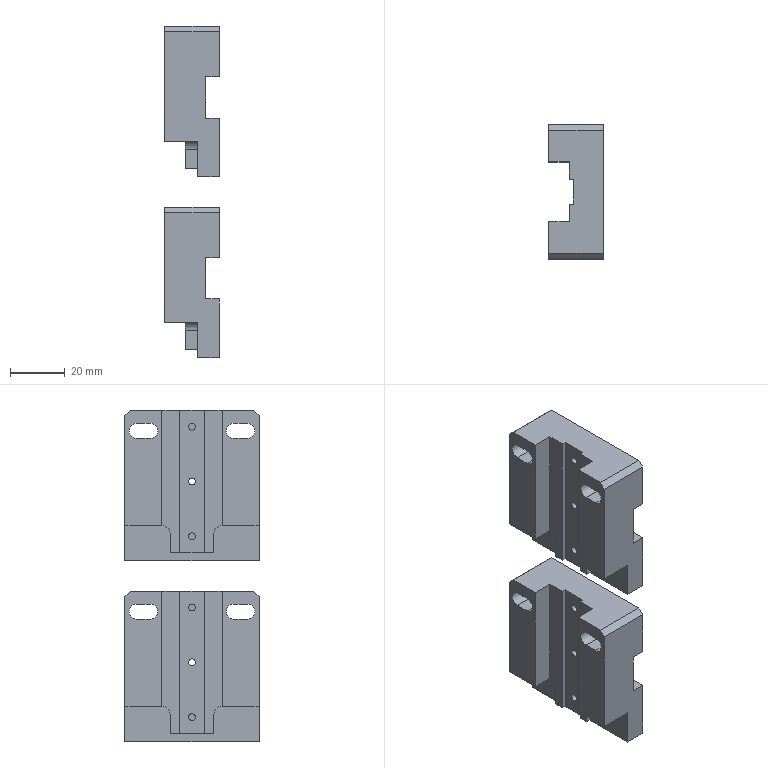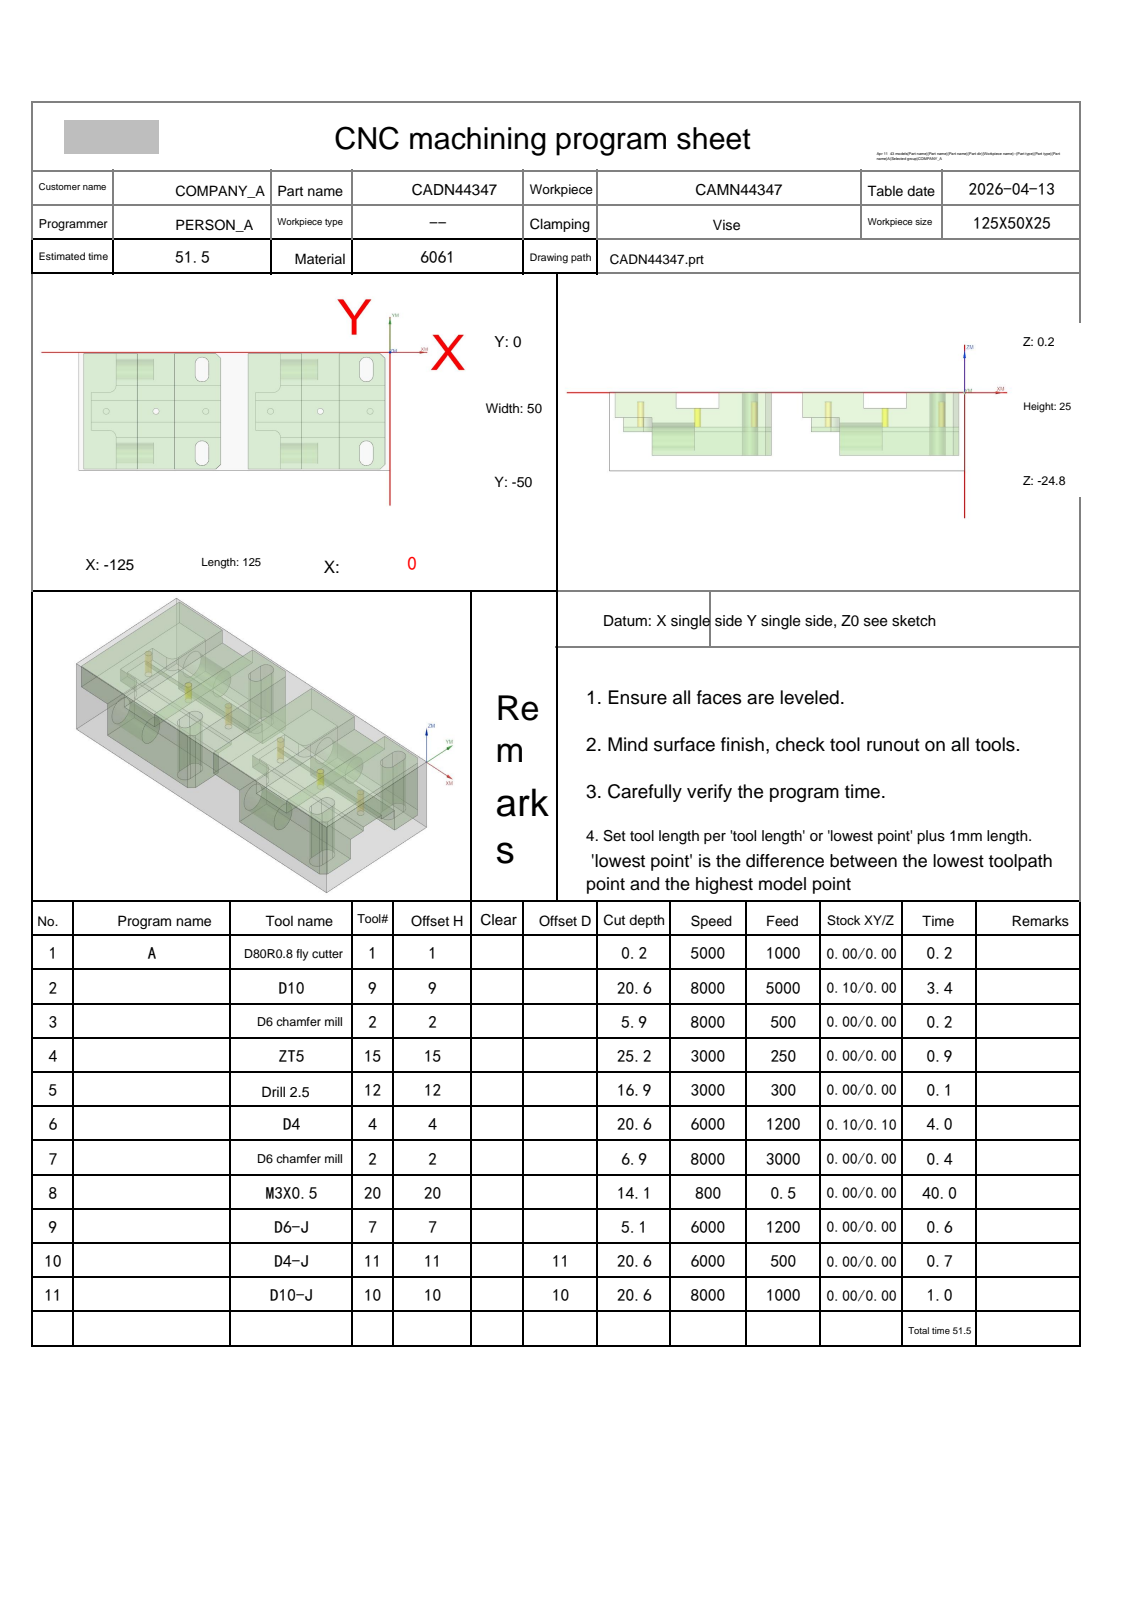NC program | NX | posted by the shop | part box 19.9 x 49 x 121 mm
Lines 1 to 1032 of 3925:
%
O0001
(Machine time: 89.70 MIN)
(===Total Tool:10===)
(T1=D80R0.8 fly cutter D=80.  R=0.8  D-  H01 Z=0.    )
(T9=D10     D=10.  R=0.   D-  H09 Z=-20.4 )
(T2=D6 chamfer mill   D=6.   R=0.   D-  H02 Z=-6.65 )
(T15=ZT5    D=5.   DR_a=118 D-  H15 Z=-25.  )
(T12=Drill 2.5  D=2.5  DR_a=118 D-  H12 Z=-16.65)
(T4=D4      D=4.   R=0.   D-  H04 Z=-20.4 )
(T20=M3X0.5 D=2.5  DR_a=180 D-  H20 Z=-13.9 )
(T7=D6-J    D=6.   R=0.   D7  H07 Z=-4.9  )
(T11=D4-J   D=4.   R=0.   D11 H11 Z=-20.4 )
(T10=D10-J  D=10.  R=0.   D10 H10 Z=-20.4 )
G80 G90 G17 G49 G40
G91 G28 Z0
M01
N1 T01 M06
(D80R0.8 fly cutter  D=80. R=0.8 H=01 ce=0.00 di=0.00)
G00 G90 G54 X43. Y-25. M03 S5000
G43 H01 Z20.
M08
Z2.
G01 Z0.0 F1000.
X38.
X-163.
X-168.
Z2.
G00 Z20.
G91 G28 Z0.0
M05
M09
G91 G28 Z0.0
M01
N2 T09 M06
(D10  D=10. R=0. H=09 ce=0.10 di=0.00)
G00 G90 G54 X-96.5 Y4.6 M03 S8000
G43 H09 Z20.
M08
Z.5
G01 X-70. Z.414 F5000.
G02 X-66.394 Y3.106 Z.401 I0.0 J-5.1
G01 X-64.394 Y1.106 Z.391
G02 X-62.9 Y-2.5 Z.378 I-3.606 J-3.606
G01 Y-47.5 Z.232
G02 X-64.394 Y-51.106 Z.219 I-5.1 J0.0
G01 X-66.394 Y-53.106 Z.21
G02 X-70. Y-54.6 Z.197 I-3.606 J3.606
G01 X-123. Z.024
G02 X-128.1 Y-49.5 Z-.002 I0.0 J5.1
G01 Y-.5 Z-.162
G02 X-123. Y4.6 Z-.188 I5.1 J0.0
G01 X-70. Z-.36
G02 X-66.394 Y3.106 Z-.373 I0.0 J-5.1
G01 X-64.394 Y1.106 Z-.383
G02 X-62.9 Y-2.5 Z-.396 I-3.606 J-3.606
G01 Y-47.5 Z-.542
G02 X-64.394 Y-51.106 Z-.555 I-5.1 J0.0
G01 X-66.394 Y-53.106 Z-.564
G02 X-70. Y-54.6 Z-.578 I-3.606 J3.606
G01 X-123. Z-.75
G02 X-128.1 Y-49.5 Z-.776 I0.0 J5.1
G01 Y-.5 Z-.936
G02 X-123. Y4.6 Z-.962 I5.1 J0.0
G01 X-70. Z-1.134
G02 X-66.394 Y3.106 Z-1.147 I0.0 J-5.1
G01 X-64.394 Y1.106 Z-1.157
G02 X-62.9 Y-2.5 Z-1.17 I-3.606 J-3.606
G01 Y-47.5 Z-1.316
G02 X-64.394 Y-51.106 Z-1.329 I-5.1 J0.0
G01 X-66.394 Y-53.106 Z-1.339
G02 X-70. Y-54.6 Z-1.352 I-3.606 J3.606
G01 X-123. Z-1.524
G02 X-128.1 Y-49.5 Z-1.55 I0.0 J5.1
G01 Y-.5 Z-1.71
G02 X-123. Y4.6 Z-1.736 I5.1 J0.0
G01 X-70. Z-1.909
G02 X-66.394 Y3.106 Z-1.922 I0.0 J-5.1
G01 X-64.394 Y1.106 Z-1.931
G02 X-62.9 Y-2.5 Z-1.944 I-3.606 J-3.606
G01 Y-47.5 Z-2.09
G02 X-64.394 Y-51.106 Z-2.103 I-5.1 J0.0
G01 X-66.394 Y-53.106 Z-2.113
G02 X-70. Y-54.6 Z-2.126 I-3.606 J3.606
G01 X-123. Z-2.298
G02 X-128.1 Y-49.5 Z-2.324 I0.0 J5.1
G01 Y-.5 Z-2.484
G02 X-123. Y4.6 Z-2.51 I5.1 J0.0
G01 X-70. Z-2.683
G02 X-66.394 Y3.106 Z-2.696 I0.0 J-5.1
G01 X-64.394 Y1.106 Z-2.705
G02 X-62.9 Y-2.5 Z-2.718 I-3.606 J-3.606
G01 Y-47.5 Z-2.864
G02 X-64.394 Y-51.106 Z-2.877 I-5.1 J0.0
G01 X-66.394 Y-53.106 Z-2.887
G02 X-70. Y-54.6 Z-2.9 I-3.606 J3.606
G01 X-123. Z-3.072
G02 X-128.1 Y-49.5 Z-3.098 I0.0 J5.1
G01 Y-.5 Z-3.258
G02 X-123. Y4.6 Z-3.284 I5.1 J0.0
G01 X-70. Z-3.457
G02 X-66.394 Y3.106 Z-3.47 I0.0 J-5.1
G01 X-64.394 Y1.106 Z-3.479
G02 X-62.9 Y-2.5 Z-3.492 I-3.606 J-3.606
G01 Y-47.5 Z-3.639
G02 X-64.394 Y-51.106 Z-3.652 I-5.1 J0.0
G01 X-66.394 Y-53.106 Z-3.661
G02 X-70. Y-54.6 Z-3.674 I-3.606 J3.606
G01 X-123. Z-3.846
G02 X-128.1 Y-49.5 Z-3.872 I0.0 J5.1
G01 Y-.5 Z-4.032
G02 X-123. Y4.6 Z-4.058 I5.1 J0.0
G01 X-70. Z-4.231
G02 X-66.394 Y3.106 Z-4.244 I0.0 J-5.1
G01 X-64.394 Y1.106 Z-4.253
G02 X-62.9 Y-2.5 Z-4.266 I-3.606 J-3.606
G01 Y-47.5 Z-4.413
G02 X-64.394 Y-51.106 Z-4.426 I-5.1 J0.0
G01 X-66.394 Y-53.106 Z-4.435
G02 X-70. Y-54.6 Z-4.448 I-3.606 J3.606
G01 X-123. Z-4.62
G02 X-128.1 Y-49.5 Z-4.647 I0.0 J5.1
G01 Y-.5 Z-4.806
G02 X-123. Y4.6 Z-4.832 I5.1 J0.0
G01 X-70. Z-5.005
G02 X-66.394 Y3.106 Z-5.018 I0.0 J-5.1
G01 X-64.394 Y1.106 Z-5.027
G02 X-62.9 Y-2.5 Z-5.04 I-3.606 J-3.606
G01 Y-47.5 Z-5.187
G02 X-64.394 Y-51.106 Z-5.2 I-5.1 J0.0
G01 X-66.394 Y-53.106 Z-5.209
G02 X-70. Y-54.6 Z-5.222 I-3.606 J3.606
G01 X-123. Z-5.395
G02 X-128.1 Y-49.5 Z-5.421 I0.0 J5.1
G01 Y-.5 Z-5.58
G02 X-123. Y4.6 Z-5.606 I5.1 J0.0
G01 X-70. Z-5.779
G02 X-66.394 Y3.106 Z-5.792 I0.0 J-5.1
G01 X-64.394 Y1.106 Z-5.801
G02 X-62.9 Y-2.5 Z-5.814 I-3.606 J-3.606
G01 Y-47.5 Z-5.961
G02 X-64.394 Y-51.106 Z-5.974 I-5.1 J0.0
G01 X-66.394 Y-53.106 Z-5.983
G02 X-70. Y-54.6 Z-5.996 I-3.606 J3.606
G01 X-123. Z-6.169
G02 X-128.1 Y-49.5 Z-6.195 I0.0 J5.1
G01 Y-.5 Z-6.354
G02 X-123. Y4.6 Z-6.38 I5.1 J0.0
G01 X-70. Z-6.553
G02 X-66.394 Y3.106 Z-6.566 I0.0 J-5.1
G01 X-64.394 Y1.106 Z-6.575
G02 X-62.9 Y-2.5 Z-6.588 I-3.606 J-3.606
G01 Y-47.5 Z-6.735
G02 X-64.394 Y-51.106 Z-6.748 I-5.1 J0.0
G01 X-66.394 Y-53.106 Z-6.757
G02 X-70. Y-54.6 Z-6.77 I-3.606 J3.606
G01 X-123. Z-6.943
G02 X-128.1 Y-49.5 Z-6.969 I0.0 J5.1
G01 Y-.5 Z-7.128
G02 X-123. Y4.6 Z-7.154 I5.1 J0.0
G01 X-70. Z-7.327
G02 X-66.394 Y3.106 Z-7.34 I0.0 J-5.1
G01 X-64.394 Y1.106 Z-7.349
G02 X-62.9 Y-2.5 Z-7.362 I-3.606 J-3.606
G01 Y-47.5 Z-7.509
G02 X-64.394 Y-51.106 Z-7.522 I-5.1 J0.0
G01 X-66.394 Y-53.106 Z-7.531
G02 X-70. Y-54.6 Z-7.544 I-3.606 J3.606
G01 X-123. Z-7.717
G02 X-128.1 Y-49.5 Z-7.743 I0.0 J5.1
G01 Y-.5 Z-7.902
G02 X-123. Y4.6 Z-7.929 I5.1 J0.0
G01 X-70. Z-8.101
G02 X-66.394 Y3.106 Z-8.114 I0.0 J-5.1
G01 X-64.394 Y1.106 Z-8.123
G02 X-62.9 Y-2.5 Z-8.136 I-3.606 J-3.606
G01 Y-47.5 Z-8.283
G02 X-64.394 Y-51.106 Z-8.296 I-5.1 J0.0
G01 X-66.394 Y-53.106 Z-8.305
G02 X-70. Y-54.6 Z-8.318 I-3.606 J3.606
G01 X-123. Z-8.491
G02 X-128.1 Y-49.5 Z-8.517 I0.0 J5.1
G01 Y-.5 Z-8.677
G02 X-123. Y4.6 Z-8.703 I5.1 J0.0
G01 X-70. Z-8.875
G02 X-66.394 Y3.106 Z-8.888 I0.0 J-5.1
G01 X-64.394 Y1.106 Z-8.897
G02 X-62.9 Y-2.5 Z-8.91 I-3.606 J-3.606
G01 Y-47.5 Z-9.057
G02 X-64.394 Y-51.106 Z-9.07 I-5.1 J0.0
G01 X-66.394 Y-53.106 Z-9.079
G02 X-70. Y-54.6 Z-9.092 I-3.606 J3.606
G01 X-123. Z-9.265
G02 X-128.1 Y-49.5 Z-9.291 I0.0 J5.1
G01 Y-.5 Z-9.451
G02 X-123. Y4.6 Z-9.477 I5.1 J0.0
G01 X-70. Z-9.649
G02 X-66.394 Y3.106 Z-9.662 I0.0 J-5.1
G01 X-64.394 Y1.106 Z-9.672
G02 X-62.9 Y-2.5 Z-9.685 I-3.606 J-3.606
G01 Y-47.5 Z-9.831
G02 X-64.394 Y-51.106 Z-9.844 I-5.1 J0.0
G01 X-66.394 Y-53.106 Z-9.853
G02 X-70. Y-54.6 Z-9.866 I-3.606 J3.606
G01 X-123. Z-10.039
G02 X-128.1 Y-49.5 Z-10.065 I0.0 J5.1
G01 Y-.5 Z-10.225
G02 X-123. Y4.6 Z-10.251 I5.1 J0.0
G01 X-70. Z-10.423
G02 X-66.394 Y3.106 Z-10.436 I0.0 J-5.1
G01 X-64.394 Y1.106 Z-10.446
G02 X-62.9 Y-2.5 Z-10.459 I-3.606 J-3.606
G01 Y-47.5 Z-10.605
G02 X-64.394 Y-51.106 Z-10.618 I-5.1 J0.0
G01 X-66.394 Y-53.106 Z-10.627
G02 X-70. Y-54.6 Z-10.64 I-3.606 J3.606
G01 X-123. Z-10.813
G02 X-128.1 Y-49.5 Z-10.839 I0.0 J5.1
G01 Y-.5 Z-10.999
G02 X-123. Y4.6 Z-11.025 I5.1 J0.0
G01 X-70. Z-11.197
G02 X-66.394 Y3.106 Z-11.21 I0.0 J-5.1
G01 X-64.394 Y1.106 Z-11.22
G02 X-62.9 Y-2.5 Z-11.233 I-3.606 J-3.606
G01 Y-47.5 Z-11.379
G02 X-64.394 Y-51.106 Z-11.392 I-5.1 J0.0
G01 X-66.394 Y-53.106 Z-11.402
G02 X-70. Y-54.6 Z-11.415 I-3.606 J3.606
G01 X-123. Z-11.587
G02 X-128.1 Y-49.5 Z-11.613 I0.0 J5.1
G01 Y-.5 Z-11.773
G02 X-123. Y4.6 Z-11.799 I5.1 J0.0
G01 X-70. Z-11.971
G02 X-66.394 Y3.106 Z-11.985 I0.0 J-5.1
G01 X-64.394 Y1.106 Z-11.994
G02 X-62.9 Y-2.5 Z-12.007 I-3.606 J-3.606
G01 Y-47.5 Z-12.153
G02 X-64.394 Y-51.106 Z-12.166 I-5.1 J0.0
G01 X-66.394 Y-53.106 Z-12.176
G02 X-70. Y-54.6 Z-12.189 I-3.606 J3.606
G01 X-123. Z-12.361
G02 X-128.1 Y-49.5 Z-12.387 I0.0 J5.1
G01 Y-.5 Z-12.547
G02 X-123. Y4.6 Z-12.573 I5.1 J0.0
G01 X-70. Z-12.746
G02 X-66.394 Y3.106 Z-12.759 I0.0 J-5.1
G01 X-64.394 Y1.106 Z-12.768
G02 X-62.9 Y-2.5 Z-12.781 I-3.606 J-3.606
G01 Y-47.5 Z-12.927
G02 X-64.394 Y-51.106 Z-12.94 I-5.1 J0.0
G01 X-66.394 Y-53.106 Z-12.95
G02 X-70. Y-54.6 Z-12.963 I-3.606 J3.606
G01 X-123. Z-13.135
G02 X-128.1 Y-49.5 Z-13.161 I0.0 J5.1
G01 Y-.5 Z-13.321
G02 X-123. Y4.6 Z-13.347 I5.1 J0.0
G01 X-70. Z-13.52
G02 X-66.394 Y3.106 Z-13.533 I0.0 J-5.1
G01 X-64.394 Y1.106 Z-13.542
G02 X-62.9 Y-2.5 Z-13.555 I-3.606 J-3.606
G01 Y-47.5 Z-13.701
G02 X-64.394 Y-51.106 Z-13.715 I-5.1 J0.0
G01 X-66.394 Y-53.106 Z-13.724
G02 X-70. Y-54.6 Z-13.737 I-3.606 J3.606
G01 X-123. Z-13.909
G02 X-128.1 Y-49.5 Z-13.935 I0.0 J5.1
G01 Y-.5 Z-14.095
G02 X-123. Y4.6 Z-14.121 I5.1 J0.0
G01 X-70. Z-14.294
G02 X-66.394 Y3.106 Z-14.307 I0.0 J-5.1
G01 X-64.394 Y1.106 Z-14.316
G02 X-62.9 Y-2.5 Z-14.329 I-3.606 J-3.606
G01 Y-47.5 Z-14.476
G02 X-64.394 Y-51.106 Z-14.489 I-5.1 J0.0
G01 X-66.394 Y-53.106 Z-14.498
G02 X-70. Y-54.6 Z-14.511 I-3.606 J3.606
G01 X-123. Z-14.683
G02 X-128.1 Y-49.5 Z-14.71 I0.0 J5.1
G01 Y-.5 Z-14.869
G02 X-123. Y4.6 Z-14.895 I5.1 J0.0
G01 X-70. Z-15.068
G02 X-66.394 Y3.106 Z-15.081 I0.0 J-5.1
G01 X-64.394 Y1.106 Z-15.09
G02 X-62.9 Y-2.5 Z-15.103 I-3.606 J-3.606
G01 Y-47.5 Z-15.25
G02 X-64.394 Y-51.106 Z-15.263 I-5.1 J0.0
G01 X-66.394 Y-53.106 Z-15.272
G02 X-70. Y-54.6 Z-15.285 I-3.606 J3.606
G01 X-123. Z-15.458
G02 X-128.1 Y-49.5 Z-15.484 I0.0 J5.1
G01 Y-.5 Z-15.643
G02 X-123. Y4.6 Z-15.669 I5.1 J0.0
G01 X-70. Z-15.842
G02 X-66.394 Y3.106 Z-15.855 I0.0 J-5.1
G01 X-64.394 Y1.106 Z-15.864
G02 X-62.9 Y-2.5 Z-15.877 I-3.606 J-3.606
G01 Y-47.5 Z-16.024
G02 X-64.394 Y-51.106 Z-16.037 I-5.1 J0.0
G01 X-66.394 Y-53.106 Z-16.046
G02 X-70. Y-54.6 Z-16.059 I-3.606 J3.606
G01 X-123. Z-16.232
G02 X-128.1 Y-49.5 Z-16.258 I0.0 J5.1
G01 Y-.5 Z-16.417
G02 X-123. Y4.6 Z-16.443 I5.1 J0.0
G01 X-70. Z-16.616
G02 X-66.394 Y3.106 Z-16.629 I0.0 J-5.1
G01 X-64.394 Y1.106 Z-16.638
G02 X-62.9 Y-2.5 Z-16.651 I-3.606 J-3.606
G01 Y-47.5 Z-16.798
G02 X-64.394 Y-51.106 Z-16.811 I-5.1 J0.0
G01 X-66.394 Y-53.106 Z-16.82
G02 X-70. Y-54.6 Z-16.833 I-3.606 J3.606
G01 X-123. Z-17.006
G02 X-128.1 Y-49.5 Z-17.032 I0.0 J5.1
G01 Y-.5 Z-17.191
G02 X-123. Y4.6 Z-17.217 I5.1 J0.0
G01 X-70. Z-17.39
G02 X-66.394 Y3.106 Z-17.403 I0.0 J-5.1
G01 X-64.394 Y1.106 Z-17.412
G02 X-62.9 Y-2.5 Z-17.425 I-3.606 J-3.606
G01 Y-47.5 Z-17.572
G02 X-64.394 Y-51.106 Z-17.585 I-5.1 J0.0
G01 X-66.394 Y-53.106 Z-17.594
G02 X-70. Y-54.6 Z-17.607 I-3.606 J3.606
G01 X-123. Z-17.78
G02 X-128.1 Y-49.5 Z-17.806 I0.0 J5.1
G01 Y-.5 Z-17.965
G02 X-123. Y4.6 Z-17.991 I5.1 J0.0
G01 X-70. Z-18.164
G02 X-66.394 Y3.106 Z-18.177 I0.0 J-5.1
G01 X-64.394 Y1.106 Z-18.186
G02 X-62.9 Y-2.5 Z-18.199 I-3.606 J-3.606
G01 Y-47.5 Z-18.346
G02 X-64.394 Y-51.106 Z-18.359 I-5.1 J0.0
G01 X-66.394 Y-53.106 Z-18.368
G02 X-70. Y-54.6 Z-18.381 I-3.606 J3.606
G01 X-123. Z-18.554
G02 X-128.1 Y-49.5 Z-18.58 I0.0 J5.1
G01 Y-.5 Z-18.739
G02 X-123. Y4.6 Z-18.766 I5.1 J0.0
G01 X-70. Z-18.938
G02 X-66.394 Y3.106 Z-18.951 I0.0 J-5.1
G01 X-64.394 Y1.106 Z-18.96
G02 X-62.9 Y-2.5 Z-18.973 I-3.606 J-3.606
G01 Y-47.5 Z-19.12
G02 X-64.394 Y-51.106 Z-19.133 I-5.1 J0.0
G01 X-66.394 Y-53.106 Z-19.142
G02 X-70. Y-54.6 Z-19.155 I-3.606 J3.606
G01 X-123. Z-19.328
G02 X-128.1 Y-49.5 Z-19.354 I0.0 J5.1
G01 Y-.5 Z-19.514
G02 X-123. Y4.6 Z-19.54 I5.1 J0.0
G01 X-70. Z-19.712
G02 X-66.394 Y3.106 Z-19.725 I0.0 J-5.1
G01 X-64.394 Y1.106 Z-19.734
G02 X-62.9 Y-2.5 Z-19.748 I-3.606 J-3.606
G01 Y-47.5 Z-19.894
G02 X-64.394 Y-51.106 Z-19.907 I-5.1 J0.0
G01 X-66.394 Y-53.106 Z-19.916
G02 X-70. Y-54.6 Z-19.929 I-3.606 J3.606
G01 X-123. Z-20.102
G02 X-128.1 Y-49.5 Z-20.128 I0.0 J5.1
G01 Y-.5 Z-20.288
G02 X-123. Y4.6 Z-20.314 I5.1 J0.0
G01 X-96.5 Z-20.4
X-70.
G02 X-66.394 Y3.106 I0.0 J-5.1
G01 X-64.394 Y1.106
G02 X-62.9 Y-2.5 I-3.606 J-3.606
G01 Y-47.5
G02 X-64.394 Y-51.106 I-5.1 J0.0
G01 X-66.394 Y-53.106
G02 X-70. Y-54.6 I-3.606 J3.606
G01 X-123.
G02 X-128.1 Y-49.5 I0.0 J5.1
G01 Y-.5
G02 X-123. Y4.6 I5.1 J0.0
G01 X-96.5
X-96.
Z-19.4
G00 Z20.
X-30.5
Z.5
G01 X-4. Z.414
G02 X-.394 Y3.106 Z.401 I0.0 J-5.1
G01 X1.606 Y1.106 Z.391
G02 X3.1 Y-2.5 Z.378 I-3.606 J-3.606
G01 Y-47.5 Z.232
G02 X1.606 Y-51.106 Z.219 I-5.1 J0.0
G01 X-.394 Y-53.106 Z.21
G02 X-4. Y-54.6 Z.197 I-3.606 J3.606
G01 X-57. Z.024
G02 X-62.1 Y-49.5 Z-.002 I0.0 J5.1
G01 Y-.5 Z-.162
G02 X-57. Y4.6 Z-.188 I5.1 J0.0
G01 X-4. Z-.36
G02 X-.394 Y3.106 Z-.373 I0.0 J-5.1
G01 X1.606 Y1.106 Z-.383
G02 X3.1 Y-2.5 Z-.396 I-3.606 J-3.606
G01 Y-47.5 Z-.542
G02 X1.606 Y-51.106 Z-.555 I-5.1 J0.0
G01 X-.394 Y-53.106 Z-.564
G02 X-4. Y-54.6 Z-.578 I-3.606 J3.606
G01 X-57. Z-.75
G02 X-62.1 Y-49.5 Z-.776 I0.0 J5.1
G01 Y-.5 Z-.936
G02 X-57. Y4.6 Z-.962 I5.1 J0.0
G01 X-4. Z-1.134
G02 X-.394 Y3.106 Z-1.147 I0.0 J-5.1
G01 X1.606 Y1.106 Z-1.157
G02 X3.1 Y-2.5 Z-1.17 I-3.606 J-3.606
G01 Y-47.5 Z-1.316
G02 X1.606 Y-51.106 Z-1.329 I-5.1 J0.0
G01 X-.394 Y-53.106 Z-1.339
G02 X-4. Y-54.6 Z-1.352 I-3.606 J3.606
G01 X-57. Z-1.524
G02 X-62.1 Y-49.5 Z-1.55 I0.0 J5.1
G01 Y-.5 Z-1.71
G02 X-57. Y4.6 Z-1.736 I5.1 J0.0
G01 X-4. Z-1.909
G02 X-.394 Y3.106 Z-1.922 I0.0 J-5.1
G01 X1.606 Y1.106 Z-1.931
G02 X3.1 Y-2.5 Z-1.944 I-3.606 J-3.606
G01 Y-47.5 Z-2.09
G02 X1.606 Y-51.106 Z-2.103 I-5.1 J0.0
G01 X-.394 Y-53.106 Z-2.113
G02 X-4. Y-54.6 Z-2.126 I-3.606 J3.606
G01 X-57. Z-2.298
G02 X-62.1 Y-49.5 Z-2.324 I0.0 J5.1
G01 Y-.5 Z-2.484
G02 X-57. Y4.6 Z-2.51 I5.1 J0.0
G01 X-4. Z-2.683
G02 X-.394 Y3.106 Z-2.696 I0.0 J-5.1
G01 X1.606 Y1.106 Z-2.705
G02 X3.1 Y-2.5 Z-2.718 I-3.606 J-3.606
G01 Y-47.5 Z-2.864
G02 X1.606 Y-51.106 Z-2.877 I-5.1 J0.0
G01 X-.394 Y-53.106 Z-2.887
G02 X-4. Y-54.6 Z-2.9 I-3.606 J3.606
G01 X-57. Z-3.072
G02 X-62.1 Y-49.5 Z-3.098 I0.0 J5.1
G01 Y-.5 Z-3.258
G02 X-57. Y4.6 Z-3.284 I5.1 J0.0
G01 X-4. Z-3.457
G02 X-.394 Y3.106 Z-3.47 I0.0 J-5.1
G01 X1.606 Y1.106 Z-3.479
G02 X3.1 Y-2.5 Z-3.492 I-3.606 J-3.606
G01 Y-47.5 Z-3.639
G02 X1.606 Y-51.106 Z-3.652 I-5.1 J0.0
G01 X-.394 Y-53.106 Z-3.661
G02 X-4. Y-54.6 Z-3.674 I-3.606 J3.606
G01 X-57. Z-3.846
G02 X-62.1 Y-49.5 Z-3.872 I0.0 J5.1
G01 Y-.5 Z-4.032
G02 X-57. Y4.6 Z-4.058 I5.1 J0.0
G01 X-4. Z-4.231
G02 X-.394 Y3.106 Z-4.244 I0.0 J-5.1
G01 X1.606 Y1.106 Z-4.253
G02 X3.1 Y-2.5 Z-4.266 I-3.606 J-3.606
G01 Y-47.5 Z-4.413
G02 X1.606 Y-51.106 Z-4.426 I-5.1 J0.0
G01 X-.394 Y-53.106 Z-4.435
G02 X-4. Y-54.6 Z-4.448 I-3.606 J3.606
G01 X-57. Z-4.62
G02 X-62.1 Y-49.5 Z-4.647 I0.0 J5.1
G01 Y-.5 Z-4.806
G02 X-57. Y4.6 Z-4.832 I5.1 J0.0
G01 X-4. Z-5.005
G02 X-.394 Y3.106 Z-5.018 I0.0 J-5.1
G01 X1.606 Y1.106 Z-5.027
G02 X3.1 Y-2.5 Z-5.04 I-3.606 J-3.606
G01 Y-47.5 Z-5.187
G02 X1.606 Y-51.106 Z-5.2 I-5.1 J0.0
G01 X-.394 Y-53.106 Z-5.209
G02 X-4. Y-54.6 Z-5.222 I-3.606 J3.606
G01 X-57. Z-5.395
G02 X-62.1 Y-49.5 Z-5.421 I0.0 J5.1
G01 Y-.5 Z-5.58
G02 X-57. Y4.6 Z-5.606 I5.1 J0.0
G01 X-4. Z-5.779
G02 X-.394 Y3.106 Z-5.792 I0.0 J-5.1
G01 X1.606 Y1.106 Z-5.801
G02 X3.1 Y-2.5 Z-5.814 I-3.606 J-3.606
G01 Y-47.5 Z-5.961
G02 X1.606 Y-51.106 Z-5.974 I-5.1 J0.0
G01 X-.394 Y-53.106 Z-5.983
G02 X-4. Y-54.6 Z-5.996 I-3.606 J3.606
G01 X-57. Z-6.169
G02 X-62.1 Y-49.5 Z-6.195 I0.0 J5.1
G01 Y-.5 Z-6.354
G02 X-57. Y4.6 Z-6.38 I5.1 J0.0
G01 X-4. Z-6.553
G02 X-.394 Y3.106 Z-6.566 I0.0 J-5.1
G01 X1.606 Y1.106 Z-6.575
G02 X3.1 Y-2.5 Z-6.588 I-3.606 J-3.606
G01 Y-47.5 Z-6.735
G02 X1.606 Y-51.106 Z-6.748 I-5.1 J0.0
G01 X-.394 Y-53.106 Z-6.757
G02 X-4. Y-54.6 Z-6.77 I-3.606 J3.606
G01 X-57. Z-6.943
G02 X-62.1 Y-49.5 Z-6.969 I0.0 J5.1
G01 Y-.5 Z-7.128
G02 X-57. Y4.6 Z-7.154 I5.1 J0.0
G01 X-4. Z-7.327
G02 X-.394 Y3.106 Z-7.34 I0.0 J-5.1
G01 X1.606 Y1.106 Z-7.349
G02 X3.1 Y-2.5 Z-7.362 I-3.606 J-3.606
G01 Y-47.5 Z-7.509
G02 X1.606 Y-51.106 Z-7.522 I-5.1 J0.0
G01 X-.394 Y-53.106 Z-7.531
G02 X-4. Y-54.6 Z-7.544 I-3.606 J3.606
G01 X-57. Z-7.717
G02 X-62.1 Y-49.5 Z-7.743 I0.0 J5.1
G01 Y-.5 Z-7.902
G02 X-57. Y4.6 Z-7.929 I5.1 J0.0
G01 X-4. Z-8.101
G02 X-.394 Y3.106 Z-8.114 I0.0 J-5.1
G01 X1.606 Y1.106 Z-8.123
G02 X3.1 Y-2.5 Z-8.136 I-3.606 J-3.606
G01 Y-47.5 Z-8.283
G02 X1.606 Y-51.106 Z-8.296 I-5.1 J0.0
G01 X-.394 Y-53.106 Z-8.305
G02 X-4. Y-54.6 Z-8.318 I-3.606 J3.606
G01 X-57. Z-8.491
G02 X-62.1 Y-49.5 Z-8.517 I0.0 J5.1
G01 Y-.5 Z-8.677
G02 X-57. Y4.6 Z-8.703 I5.1 J0.0
G01 X-4. Z-8.875
G02 X-.394 Y3.106 Z-8.888 I0.0 J-5.1
G01 X1.606 Y1.106 Z-8.897
G02 X3.1 Y-2.5 Z-8.91 I-3.606 J-3.606
G01 Y-47.5 Z-9.057
G02 X1.606 Y-51.106 Z-9.07 I-5.1 J0.0
G01 X-.394 Y-53.106 Z-9.079
G02 X-4. Y-54.6 Z-9.092 I-3.606 J3.606
G01 X-57. Z-9.265
G02 X-62.1 Y-49.5 Z-9.291 I0.0 J5.1
G01 Y-.5 Z-9.451
G02 X-57. Y4.6 Z-9.477 I5.1 J0.0
G01 X-4. Z-9.649
G02 X-.394 Y3.106 Z-9.662 I0.0 J-5.1
G01 X1.606 Y1.106 Z-9.672
G02 X3.1 Y-2.5 Z-9.685 I-3.606 J-3.606
G01 Y-47.5 Z-9.831
G02 X1.606 Y-51.106 Z-9.844 I-5.1 J0.0
G01 X-.394 Y-53.106 Z-9.853
G02 X-4. Y-54.6 Z-9.866 I-3.606 J3.606
G01 X-57. Z-10.039
G02 X-62.1 Y-49.5 Z-10.065 I0.0 J5.1
G01 Y-.5 Z-10.225
G02 X-57. Y4.6 Z-10.251 I5.1 J0.0
G01 X-4. Z-10.423
G02 X-.394 Y3.106 Z-10.436 I0.0 J-5.1
G01 X1.606 Y1.106 Z-10.446
G02 X3.1 Y-2.5 Z-10.459 I-3.606 J-3.606
G01 Y-47.5 Z-10.605
G02 X1.606 Y-51.106 Z-10.618 I-5.1 J0.0
G01 X-.394 Y-53.106 Z-10.627
G02 X-4. Y-54.6 Z-10.64 I-3.606 J3.606
G01 X-57. Z-10.813
G02 X-62.1 Y-49.5 Z-10.839 I0.0 J5.1
G01 Y-.5 Z-10.999
G02 X-57. Y4.6 Z-11.025 I5.1 J0.0
G01 X-4. Z-11.197
G02 X-.394 Y3.106 Z-11.21 I0.0 J-5.1
G01 X1.606 Y1.106 Z-11.22
G02 X3.1 Y-2.5 Z-11.233 I-3.606 J-3.606
G01 Y-47.5 Z-11.379
G02 X1.606 Y-51.106 Z-11.392 I-5.1 J0.0
G01 X-.394 Y-53.106 Z-11.402
G02 X-4. Y-54.6 Z-11.415 I-3.606 J3.606
G01 X-57. Z-11.587
G02 X-62.1 Y-49.5 Z-11.613 I0.0 J5.1
G01 Y-.5 Z-11.773
G02 X-57. Y4.6 Z-11.799 I5.1 J0.0
G01 X-4. Z-11.971
G02 X-.394 Y3.106 Z-11.985 I0.0 J-5.1
G01 X1.606 Y1.106 Z-11.994
G02 X3.1 Y-2.5 Z-12.007 I-3.606 J-3.606
G01 Y-47.5 Z-12.153
G02 X1.606 Y-51.106 Z-12.166 I-5.1 J0.0
G01 X-.394 Y-53.106 Z-12.176
G02 X-4. Y-54.6 Z-12.189 I-3.606 J3.606
G01 X-57. Z-12.361
G02 X-62.1 Y-49.5 Z-12.387 I0.0 J5.1
G01 Y-.5 Z-12.547
G02 X-57. Y4.6 Z-12.573 I5.1 J0.0
G01 X-4. Z-12.746
G02 X-.394 Y3.106 Z-12.759 I0.0 J-5.1
G01 X1.606 Y1.106 Z-12.768
G02 X3.1 Y-2.5 Z-12.781 I-3.606 J-3.606
G01 Y-47.5 Z-12.927
G02 X1.606 Y-51.106 Z-12.94 I-5.1 J0.0
G01 X-.394 Y-53.106 Z-12.95
G02 X-4. Y-54.6 Z-12.963 I-3.606 J3.606
G01 X-57. Z-13.135
G02 X-62.1 Y-49.5 Z-13.161 I0.0 J5.1
G01 Y-.5 Z-13.321
G02 X-57. Y4.6 Z-13.347 I5.1 J0.0
G01 X-4. Z-13.52
G02 X-.394 Y3.106 Z-13.533 I0.0 J-5.1
G01 X1.606 Y1.106 Z-13.542
G02 X3.1 Y-2.5 Z-13.555 I-3.606 J-3.606
G01 Y-47.5 Z-13.701
G02 X1.606 Y-51.106 Z-13.715 I-5.1 J0.0
G01 X-.394 Y-53.106 Z-13.724
G02 X-4. Y-54.6 Z-13.737 I-3.606 J3.606
G01 X-57. Z-13.909
G02 X-62.1 Y-49.5 Z-13.935 I0.0 J5.1
G01 Y-.5 Z-14.095
G02 X-57. Y4.6 Z-14.121 I5.1 J0.0
G01 X-4. Z-14.294
G02 X-.394 Y3.106 Z-14.307 I0.0 J-5.1
G01 X1.606 Y1.106 Z-14.316
G02 X3.1 Y-2.5 Z-14.329 I-3.606 J-3.606
G01 Y-47.5 Z-14.476
G02 X1.606 Y-51.106 Z-14.489 I-5.1 J0.0
G01 X-.394 Y-53.106 Z-14.498
G02 X-4. Y-54.6 Z-14.511 I-3.606 J3.606
G01 X-57. Z-14.683
G02 X-62.1 Y-49.5 Z-14.71 I0.0 J5.1
G01 Y-.5 Z-14.869
G02 X-57. Y4.6 Z-14.895 I5.1 J0.0
G01 X-4. Z-15.068
G02 X-.394 Y3.106 Z-15.081 I0.0 J-5.1
G01 X1.606 Y1.106 Z-15.09
G02 X3.1 Y-2.5 Z-15.103 I-3.606 J-3.606
G01 Y-47.5 Z-15.25
G02 X1.606 Y-51.106 Z-15.263 I-5.1 J0.0
G01 X-.394 Y-53.106 Z-15.272
G02 X-4. Y-54.6 Z-15.285 I-3.606 J3.606
G01 X-57. Z-15.458
G02 X-62.1 Y-49.5 Z-15.484 I0.0 J5.1
G01 Y-.5 Z-15.643
G02 X-57. Y4.6 Z-15.669 I5.1 J0.0
G01 X-4. Z-15.842
G02 X-.394 Y3.106 Z-15.855 I0.0 J-5.1
G01 X1.606 Y1.106 Z-15.864
G02 X3.1 Y-2.5 Z-15.877 I-3.606 J-3.606
G01 Y-47.5 Z-16.024
G02 X1.606 Y-51.106 Z-16.037 I-5.1 J0.0
G01 X-.394 Y-53.106 Z-16.046
G02 X-4. Y-54.6 Z-16.059 I-3.606 J3.606
G01 X-57. Z-16.232
G02 X-62.1 Y-49.5 Z-16.258 I0.0 J5.1
G01 Y-.5 Z-16.417
G02 X-57. Y4.6 Z-16.443 I5.1 J0.0
G01 X-4. Z-16.616
G02 X-.394 Y3.106 Z-16.629 I0.0 J-5.1
G01 X1.606 Y1.106 Z-16.638
G02 X3.1 Y-2.5 Z-16.651 I-3.606 J-3.606
G01 Y-47.5 Z-16.798
G02 X1.606 Y-51.106 Z-16.811 I-5.1 J0.0
G01 X-.394 Y-53.106 Z-16.82
G02 X-4. Y-54.6 Z-16.833 I-3.606 J3.606
G01 X-57. Z-17.006
G02 X-62.1 Y-49.5 Z-17.032 I0.0 J5.1
G01 Y-.5 Z-17.191
G02 X-57. Y4.6 Z-17.217 I5.1 J0.0
G01 X-4. Z-17.39
G02 X-.394 Y3.106 Z-17.403 I0.0 J-5.1
G01 X1.606 Y1.106 Z-17.412
G02 X3.1 Y-2.5 Z-17.425 I-3.606 J-3.606
G01 Y-47.5 Z-17.572
G02 X1.606 Y-51.106 Z-17.585 I-5.1 J0.0
G01 X-.394 Y-53.106 Z-17.594
G02 X-4. Y-54.6 Z-17.607 I-3.606 J3.606
G01 X-57. Z-17.78
G02 X-62.1 Y-49.5 Z-17.806 I0.0 J5.1
G01 Y-.5 Z-17.965
G02 X-57. Y4.6 Z-17.991 I5.1 J0.0
G01 X-4. Z-18.164
G02 X-.394 Y3.106 Z-18.177 I0.0 J-5.1
G01 X1.606 Y1.106 Z-18.186
G02 X3.1 Y-2.5 Z-18.199 I-3.606 J-3.606
G01 Y-47.5 Z-18.346
G02 X1.606 Y-51.106 Z-18.359 I-5.1 J0.0
G01 X-.394 Y-53.106 Z-18.368
G02 X-4. Y-54.6 Z-18.381 I-3.606 J3.606
G01 X-57. Z-18.554
G02 X-62.1 Y-49.5 Z-18.58 I0.0 J5.1
G01 Y-.5 Z-18.739
G02 X-57. Y4.6 Z-18.766 I5.1 J0.0
G01 X-4. Z-18.938
G02 X-.394 Y3.106 Z-18.951 I0.0 J-5.1
G01 X1.606 Y1.106 Z-18.96
G02 X3.1 Y-2.5 Z-18.973 I-3.606 J-3.606
G01 Y-47.5 Z-19.12
G02 X1.606 Y-51.106 Z-19.133 I-5.1 J0.0
G01 X-.394 Y-53.106 Z-19.142
G02 X-4. Y-54.6 Z-19.155 I-3.606 J3.606
G01 X-57. Z-19.328
G02 X-62.1 Y-49.5 Z-19.354 I0.0 J5.1
G01 Y-.5 Z-19.514
G02 X-57. Y4.6 Z-19.54 I5.1 J0.0
G01 X-4. Z-19.712
G02 X-.394 Y3.106 Z-19.725 I0.0 J-5.1
G01 X1.606 Y1.106 Z-19.734
G02 X3.1 Y-2.5 Z-19.748 I-3.606 J-3.606
G01 Y-47.5 Z-19.894
G02 X1.606 Y-51.106 Z-19.907 I-5.1 J0.0
G01 X-.394 Y-53.106 Z-19.916
G02 X-4. Y-54.6 Z-19.929 I-3.606 J3.606
G01 X-57. Z-20.102
G02 X-62.1 Y-49.5 Z-20.128 I0.0 J5.1
G01 Y-.5 Z-20.288
G02 X-57. Y4.6 Z-20.314 I5.1 J0.0
G01 X-30.5 Z-20.4
X-4.
G02 X-.394 Y3.106 I0.0 J-5.1
G01 X1.606 Y1.106
G02 X3.1 Y-2.5 I-3.606 J-3.606
G01 Y-47.5
G02 X1.606 Y-51.106 I-5.1 J0.0
G01 X-.394 Y-53.106
G02 X-4. Y-54.6 I-3.606 J3.606
G01 X-57.
G02 X-62.1 Y-49.5 I0.0 J5.1
G01 Y-.5
G02 X-57. Y4.6 I5.1 J0.0
G01 X-30.5
X-30.
Z-19.4
G00 Z20.
G00 G90 X-94. Y-57.6 M03 S6000
Z20.
Z.02
G01 Z-.48 F3500.
Y-50.5
X-91.55
Y.5
X-96.45
Y-50.5
X-94.
X-93.5
Z.02
G00 Z.5
X-94. Y-57.6
Z-.46
G01 Z-.96
Y-50.5
X-91.55
Y.5
X-96.45
Y-50.5
X-94.
X-93.5
Z-.46
G00 Z.02
X-94. Y-57.6
Z-.94
G01 Z-1.44
Y-50.5
X-91.55
Y.5
X-96.45
Y-50.5
X-94.
X-93.5
Z-.94
G00 Z-.46
X-94. Y-57.6
Z-1.42
G01 Z-1.92
Y-50.5
X-91.55
Y.5
X-96.45
Y-50.5
X-94.
X-93.5
Z-1.42
G00 Z-.94
X-94. Y-57.6
Z-1.9
G01 Z-2.4
Y-50.5
X-91.55
Y.5
X-96.45
Y-50.5
X-94.
X-93.5
Z-1.9
G00 Z-1.42
X-94. Y-57.6
Z-2.38
G01 Z-2.88
Y-50.5
X-91.55
Y.5
X-96.45
Y-50.5
X-94.
X-93.5
Z-2.38
G00 Z-1.9
X-94. Y-57.6
Z-2.86
G01 Z-3.36
Y-50.5
X-91.55
Y.5
X-96.45
Y-50.5
X-94.
X-93.5
Z-2.86
G00 Z-2.38
X-94. Y-57.6
Z-3.34
G01 Z-3.84
Y-50.5
X-91.55
Y.5
X-96.45
Y-50.5
X-94.
X-93.5
Z-3.34
G00 Z-2.86
X-94. Y-57.6
Z-3.82
G01 Z-4.32
Y-50.5
X-91.55
Y.5
X-96.45
Y-50.5
X-94.
X-93.5
Z-3.82
G00 Z-3.34
X-94. Y-57.6
Z-4.3
G01 Z-4.8
Y-50.5
X-91.55
Y.5
X-96.45
Y-50.5
X-94.
X-93.5
Z-4.3
G00 Z20.
X-28. Y-57.6
Z.02
G01 Z-.48
Y-50.5
X-25.55
Y.5
X-30.45
Y-50.5
X-28.
X-27.5
Z.02
G00 Z.5
X-28. Y-57.6
Z-.46
G01 Z-.96
Y-50.5
X-25.55
Y.5
X-30.45
Y-50.5
X-28.
X-27.5
Z-.46
G00 Z.02
X-28. Y-57.6
Z-.94
G01 Z-1.44
Y-50.5
X-25.55
Y.5
X-30.45
Y-50.5
X-28.
X-27.5
Z-.94
G00 Z-.46
X-28. Y-57.6
Z-1.42
G01 Z-1.92
Y-50.5
X-25.55
Y.5
X-30.45
Y-50.5
X-28.
X-27.5
Z-1.42
G00 Z-.94
X-28. Y-57.6
Z-1.9
G01 Z-2.4
Y-50.5
X-25.55
Y.5
X-30.45
Y-50.5
X-28.
X-27.5
Z-1.9
G00 Z-1.42
X-28. Y-57.6
Z-2.38
G01 Z-2.88
Y-50.5
X-25.55
Y.5
X-30.45
Y-50.5
X-28.
X-27.5
Z-2.38
G00 Z-1.9
X-28. Y-57.6
Z-2.86
G01 Z-3.36
Y-50.5
X-25.55
Y.5
X-30.45
Y-50.5
X-28.
X-27.5
Z-2.86
G00 Z-2.38
X-28. Y-57.6
Z-3.34
G01 Z-3.84
Y-50.5
X-25.55
Y.5
X-30.45
Y-50.5
X-28.
X-27.5
Z-3.34
G00 Z-2.86
X-28. Y-57.6
Z-3.82
G01 Z-4.32
Y-50.5
X-25.55
Y.5
X-30.45
Y-50.5
X-28.
X-27.5
Z-3.82
G00 Z-3.34
X-28. Y-57.6
Z-4.3
G01 Z-4.8
Y-50.5
X-25.55
Y.5
X-30.45
Y-50.5
X-28.
X-27.5
Z-4.3
G00 Z20.
G91 G28 Z0.0
M05
M09
G91 G28 Z0.0
M01
N3 T02 M06
(D6 chamfer mill  D=6. R=0. H=02 ce=0.00 di=0.10)
G00 G90 G54 X-28. Y-25. M03 S8000
G43 H02 Z20.
M08
G98 G81 X-28. Y-25. Z-5.7 R-3.9 F500.
X-94.
G80
G00 Z20.
G00 G90 X-75.5 Y-4.75 M03 S3000
Z20.
G98 G81 X-75.5 Y-4.75 Z-1.55 R1. F200.
X-9.5
X-75.5 Y-9.75
X-9.5
X-75.5 Y-40.25
X-9.5
X-75.5 Y-45.25
X-9.5
G80
G00 Z20.
G91 G28 Z0.0
M05
M09
G91 G28 Z0.0
M01
N4 T15 M06
(ZT5 D=5. DR_a=118 H=15)
G00 G90 G54 X-75.5 Y-4.75 M03 S3000
G43 H15 Z20.
M08
G98 G83 X-75.5 Y-4.75 Z-25. R1. F250. Q3.
X-9.5
X-75.5 Y-9.75
X-9.5
X-75.5 Y-40.25
X-9.5
X-75.5 Y-45.25
X-9.5
G80
G00 Z20.
G91 G28 Z0.0
M05
M09
G91 G28 Z0.0
M01
N5 T12 M06
(Drill 2.5 D=2.5 DR_a=118 H=12)
G00 G90 G54 X-28. Y-25. M03 S3000
G43 H12 Z20.
M08
G98 G83 X-28. Y-25. Z-16.651 R-3.9 F300. Q2.
X-94.
G80
G00 Z20.
G91 G28 Z0.0
M05
M09
G91 G28 Z0.0
M01